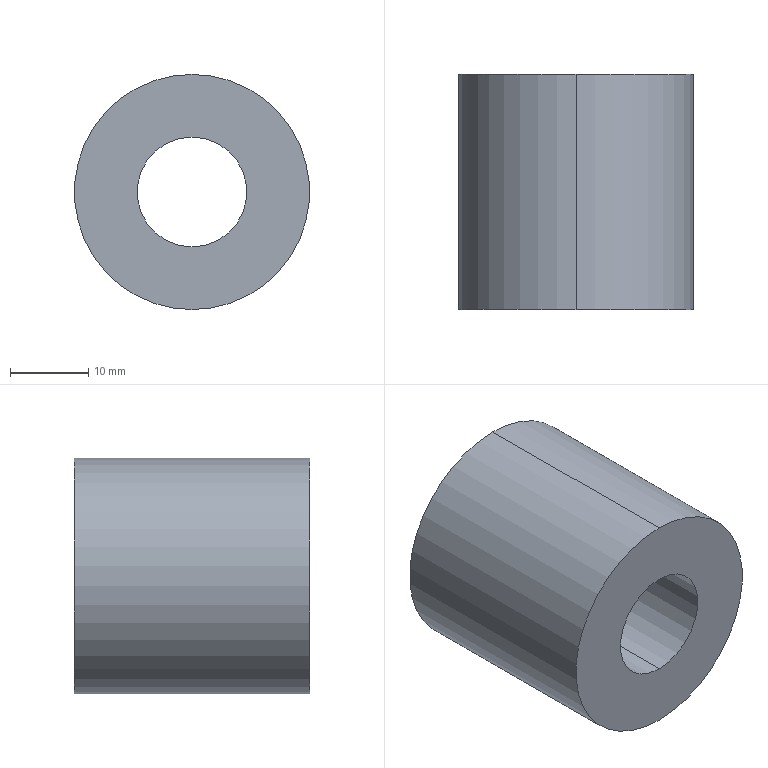Part | STEP file | inner coil2 | 1 solid | 6 faces | box 30 x 30 x 30 mm | volume 16588 mm3 | cylinder 4 | plane 2 | commonest cylinder face diameters 14 x2 30 x2
STEP:
#1=CARTESIAN_POINT('',(0.,-15.,15.));
#2=VERTEX_POINT('',#1);
#3=CARTESIAN_POINT('',(0.,-15.,-15.));
#4=VERTEX_POINT('',#3);
#5=CARTESIAN_POINT('',(0.,-15.,0.));
#6=DIRECTION('',(0.,1.,0.));
#7=DIRECTION('',(0.,0.,1.));
#8=AXIS2_PLACEMENT_3D('',#5,#6,#7);
#9=CIRCLE('',#8,15.);
#10=EDGE_CURVE('',#2,#4,#9,.T.);
#11=ORIENTED_EDGE('',*,*,#10,.T.);
#12=CARTESIAN_POINT('',(0.,15.,-15.));
#13=VERTEX_POINT('',#12);
#14=CARTESIAN_POINT('',(0.,52.348,-15.));
#15=DIRECTION('',(0.,1.,0.));
#16=VECTOR('',#15,1000.);
#17=LINE('',#14,#16);
#18=EDGE_CURVE('',#4,#13,#17,.T.);
#19=ORIENTED_EDGE('',*,*,#18,.T.);
#20=CARTESIAN_POINT('',(0.,15.,15.));
#21=VERTEX_POINT('',#20);
#22=CARTESIAN_POINT('',(0.,15.,0.));
#23=DIRECTION('',(0.,1.,0.));
#24=DIRECTION('',(0.,0.,1.));
#25=AXIS2_PLACEMENT_3D('',#22,#23,#24);
#26=CIRCLE('',#25,15.);
#27=EDGE_CURVE('',#21,#13,#26,.T.);
#28=ORIENTED_EDGE('',*,*,#27,.F.);
#29=CARTESIAN_POINT('',(0.,52.348,15.));
#30=DIRECTION('',(0.,1.,0.));
#31=VECTOR('',#30,1000.);
#32=LINE('',#29,#31);
#33=EDGE_CURVE('',#2,#21,#32,.T.);
#34=ORIENTED_EDGE('',*,*,#33,.F.);
#35=EDGE_LOOP('',(#11,#19,#28,#34));
#36=FACE_OUTER_BOUND('',#35,.T.);
#37=CARTESIAN_POINT('',(0.,52.348,0.));
#38=DIRECTION('',(0.,1.,0.));
#39=DIRECTION('',(0.,0.,1.));
#40=AXIS2_PLACEMENT_3D('',#37,#38,#39);
#41=CYLINDRICAL_SURFACE('',#40,15.);
#42=ADVANCED_FACE('',(#36),#41,.T.);
#43=CARTESIAN_POINT('',(0.,-15.,-7.));
#44=VERTEX_POINT('',#43);
#45=CARTESIAN_POINT('',(0.,-15.,7.));
#46=VERTEX_POINT('',#45);
#47=CARTESIAN_POINT('',(0.,-15.,0.));
#48=DIRECTION('',(0.,1.,0.));
#49=DIRECTION('',(0.,0.,1.));
#50=AXIS2_PLACEMENT_3D('',#47,#48,#49);
#51=CIRCLE('',#50,7.);
#52=EDGE_CURVE('',#44,#46,#51,.T.);
#53=ORIENTED_EDGE('',*,*,#52,.F.);
#54=CARTESIAN_POINT('',(0.,15.,-7.));
#55=VERTEX_POINT('',#54);
#56=CARTESIAN_POINT('',(0.,52.348,-7.));
#57=DIRECTION('',(0.,1.,0.));
#58=VECTOR('',#57,1000.);
#59=LINE('',#56,#58);
#60=EDGE_CURVE('',#44,#55,#59,.T.);
#61=ORIENTED_EDGE('',*,*,#60,.T.);
#62=CARTESIAN_POINT('',(0.,15.,7.));
#63=VERTEX_POINT('',#62);
#64=CARTESIAN_POINT('',(0.,15.,0.));
#65=DIRECTION('',(0.,1.,0.));
#66=DIRECTION('',(0.,0.,1.));
#67=AXIS2_PLACEMENT_3D('',#64,#65,#66);
#68=CIRCLE('',#67,7.);
#69=EDGE_CURVE('',#55,#63,#68,.T.);
#70=ORIENTED_EDGE('',*,*,#69,.T.);
#71=CARTESIAN_POINT('',(0.,52.348,7.));
#72=DIRECTION('',(0.,1.,0.));
#73=VECTOR('',#72,1000.);
#74=LINE('',#71,#73);
#75=EDGE_CURVE('',#46,#63,#74,.T.);
#76=ORIENTED_EDGE('',*,*,#75,.F.);
#77=EDGE_LOOP('',(#53,#61,#70,#76));
#78=FACE_OUTER_BOUND('',#77,.T.);
#79=CARTESIAN_POINT('',(0.,52.348,0.));
#80=DIRECTION('',(0.,1.,0.));
#81=DIRECTION('',(0.,0.,1.));
#82=AXIS2_PLACEMENT_3D('',#79,#80,#81);
#83=CYLINDRICAL_SURFACE('',#82,7.);
#84=ADVANCED_FACE('',(#78),#83,.F.);
#85=ORIENTED_EDGE('',*,*,#60,.F.);
#86=CARTESIAN_POINT('',(0.,-15.,0.));
#87=DIRECTION('',(0.,1.,0.));
#88=DIRECTION('',(0.,0.,1.));
#89=AXIS2_PLACEMENT_3D('',#86,#87,#88);
#90=CIRCLE('',#89,7.);
#91=EDGE_CURVE('',#46,#44,#90,.T.);
#92=ORIENTED_EDGE('',*,*,#91,.F.);
#93=ORIENTED_EDGE('',*,*,#75,.T.);
#94=CARTESIAN_POINT('',(0.,15.,0.));
#95=DIRECTION('',(0.,1.,0.));
#96=DIRECTION('',(0.,0.,1.));
#97=AXIS2_PLACEMENT_3D('',#94,#95,#96);
#98=CIRCLE('',#97,7.);
#99=EDGE_CURVE('',#63,#55,#98,.T.);
#100=ORIENTED_EDGE('',*,*,#99,.T.);
#101=EDGE_LOOP('',(#85,#92,#93,#100));
#102=FACE_OUTER_BOUND('',#101,.T.);
#103=CARTESIAN_POINT('',(0.,52.348,0.));
#104=DIRECTION('',(0.,1.,0.));
#105=DIRECTION('',(0.,0.,1.));
#106=AXIS2_PLACEMENT_3D('',#103,#104,#105);
#107=CYLINDRICAL_SURFACE('',#106,7.);
#108=ADVANCED_FACE('',(#102),#107,.F.);
#109=ORIENTED_EDGE('',*,*,#27,.T.);
#110=CARTESIAN_POINT('',(0.,15.,0.));
#111=DIRECTION('',(0.,1.,0.));
#112=DIRECTION('',(0.,0.,1.));
#113=AXIS2_PLACEMENT_3D('',#110,#111,#112);
#114=CIRCLE('',#113,15.);
#115=EDGE_CURVE('',#13,#21,#114,.T.);
#116=ORIENTED_EDGE('',*,*,#115,.T.);
#117=EDGE_LOOP('',(#109,#116));
#118=FACE_OUTER_BOUND('',#117,.T.);
#119=ORIENTED_EDGE('',*,*,#99,.F.);
#120=ORIENTED_EDGE('',*,*,#69,.F.);
#121=EDGE_LOOP('',(#119,#120));
#122=FACE_BOUND('',#121,.T.);
#123=CARTESIAN_POINT('',(-15.,15.,0.));
#124=DIRECTION('',(0.,1.,0.));
#125=DIRECTION('',(0.,0.,1.));
#126=AXIS2_PLACEMENT_3D('',#123,#124,#125);
#127=PLANE('',#126);
#128=ADVANCED_FACE('',(#118,#122),#127,.T.);
#129=ORIENTED_EDGE('',*,*,#18,.F.);
#130=CARTESIAN_POINT('',(0.,-15.,0.));
#131=DIRECTION('',(0.,1.,0.));
#132=DIRECTION('',(0.,0.,1.));
#133=AXIS2_PLACEMENT_3D('',#130,#131,#132);
#134=CIRCLE('',#133,15.);
#135=EDGE_CURVE('',#4,#2,#134,.T.);
#136=ORIENTED_EDGE('',*,*,#135,.T.);
#137=ORIENTED_EDGE('',*,*,#33,.T.);
#138=ORIENTED_EDGE('',*,*,#115,.F.);
#139=EDGE_LOOP('',(#129,#136,#137,#138));
#140=FACE_OUTER_BOUND('',#139,.T.);
#141=CARTESIAN_POINT('',(0.,52.348,0.));
#142=DIRECTION('',(0.,1.,0.));
#143=DIRECTION('',(0.,0.,1.));
#144=AXIS2_PLACEMENT_3D('',#141,#142,#143);
#145=CYLINDRICAL_SURFACE('',#144,15.);
#146=ADVANCED_FACE('',(#140),#145,.T.);
#147=ORIENTED_EDGE('',*,*,#91,.T.);
#148=ORIENTED_EDGE('',*,*,#52,.T.);
#149=EDGE_LOOP('',(#147,#148));
#150=FACE_BOUND('',#149,.T.);
#151=ORIENTED_EDGE('',*,*,#10,.F.);
#152=ORIENTED_EDGE('',*,*,#135,.F.);
#153=EDGE_LOOP('',(#151,#152));
#154=FACE_OUTER_BOUND('',#153,.T.);
#155=CARTESIAN_POINT('',(-15.,-15.,0.));
#156=DIRECTION('',(0.,-1.,0.));
#157=DIRECTION('',(0.,0.,-1.));
#158=AXIS2_PLACEMENT_3D('',#155,#156,#157);
#159=PLANE('',#158);
#160=ADVANCED_FACE('',(#150,#154),#159,.T.);
#161=CLOSED_SHELL('',(#42,#84,#108,#128,#146,#160));
#162=MANIFOLD_SOLID_BREP('',#161);
#163=CARTESIAN_POINT('',(0.,0.,0.));
#164=DIRECTION('',(0.,0.,1.));
#165=DIRECTION('',(1.,0.,0.));
#166=AXIS2_PLACEMENT_3D('',#163,#164,#165);
#167=(LENGTH_UNIT()NAMED_UNIT(*)SI_UNIT(.MILLI.,.METRE.));
#168=UNCERTAINTY_MEASURE_WITH_UNIT(LENGTH_MEASURE(0.00001),#167,'','');
#169=(NAMED_UNIT(*)PLANE_ANGLE_UNIT()SI_UNIT($,.RADIAN.));
#170=(NAMED_UNIT(*)SI_UNIT($,.STERADIAN.)SOLID_ANGLE_UNIT());
#171=(GEOMETRIC_REPRESENTATION_CONTEXT(3)GLOBAL_UNCERTAINTY_ASSIGNED_CONTEXT((#168))GLOBAL_UNIT_ASSIGNED_CONTEXT((#167,#169,#170))REPRESENTATION_CONTEXT('',''));
#172=ADVANCED_BREP_SHAPE_REPRESENTATION('',(#162,#166),#171);